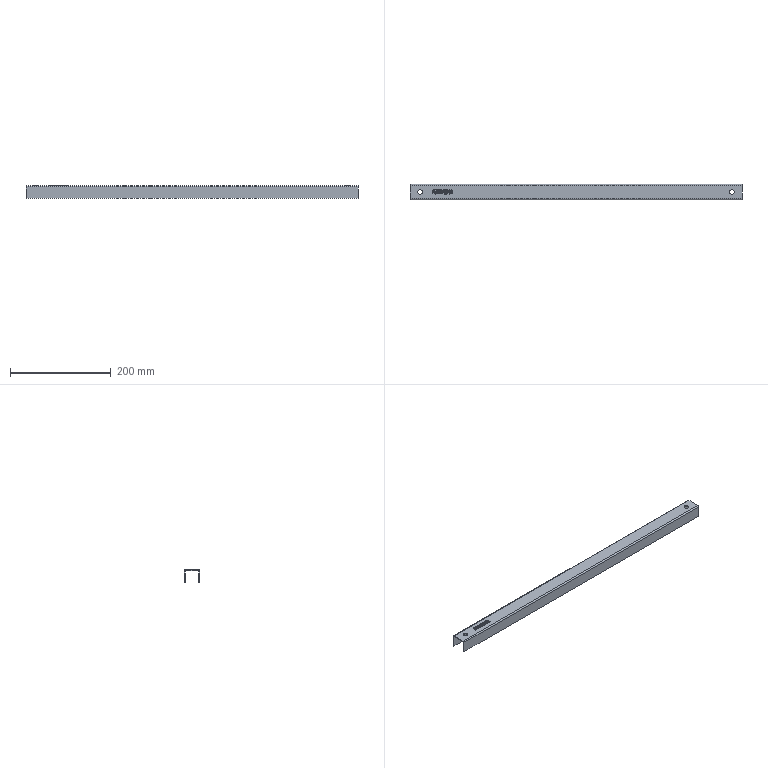Part | STEP file | Electrical Cabinet Base Plate Rib | 1 solid | 275 faces | box 660 x 30 x 25 mm | volume 98224 mm3 | plane 156 | spline 111 | cylinder 8 | commonest cylinder face diameters 9 x4 1 x2 5 x2